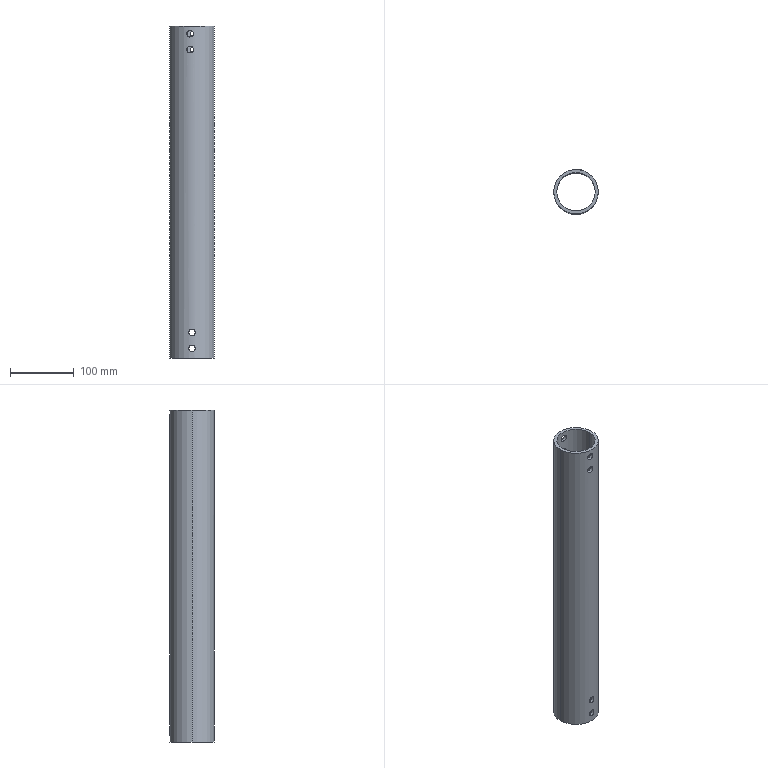Part | SolidWorks | features MirrorStock 1 | 1 solid | 22 faces | box 70 x 70 x 520 mm | volume 527553 mm3 | cylinder 20 | plane 2 | commonest cylinder face diameters 10.2 x8 10.5 x8 60 x2 70 x2